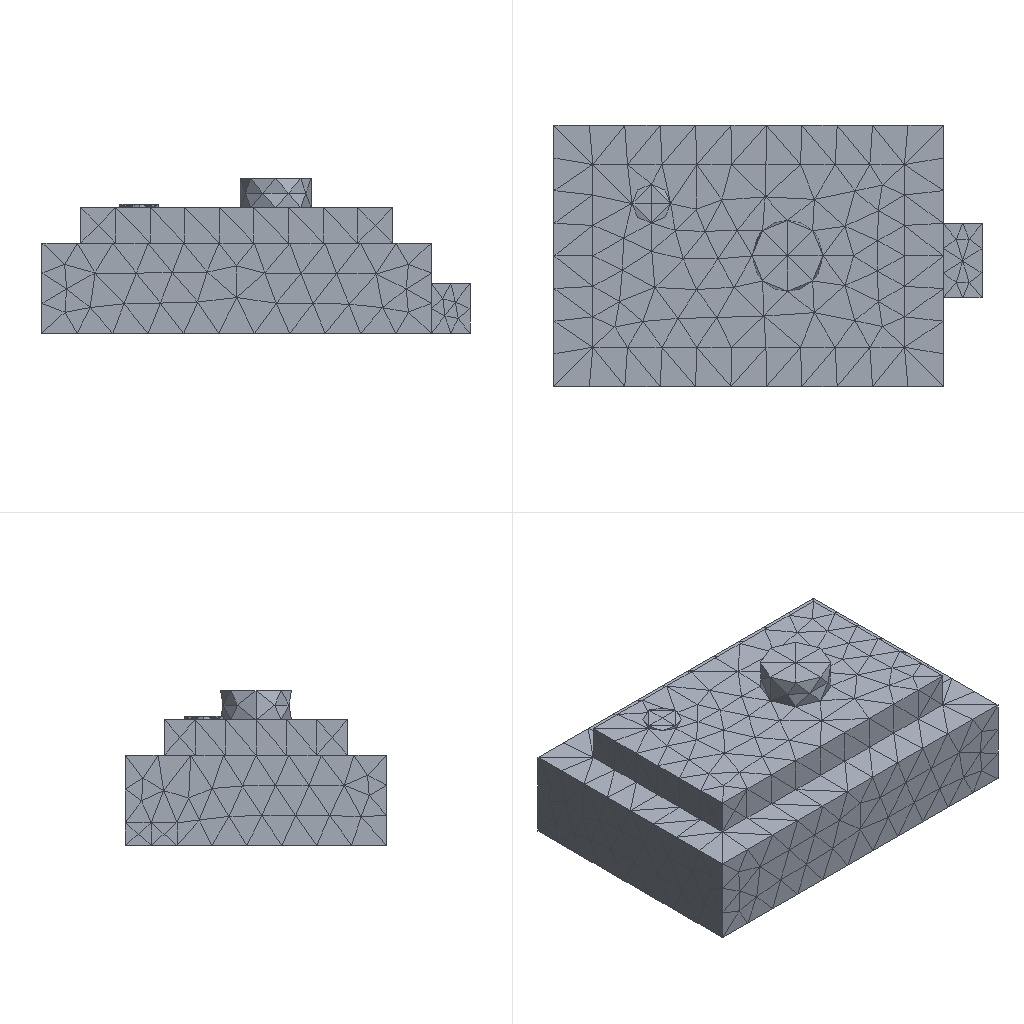Simulation study | ansys mapdl
Set-up summary:
category,name,step,type,value,unit,region
solver,ansys_mapdl
units,mm-N-s-tonne (MPa),,inferred,E=210000 density=
analysis,model,,static
mesh,nodes,,,4806
mesh,elements,,,2881
element_type,SOLID187,,,2881
material,mat 1,,E,210000
material,mat 1,,nu,0.3
load,,model,body load temp,,,all
load,,model,force,"1000 [dir=(0, 0, -1) n=142]",,node list
bc,,model,fixed,"[dofs=UX,UY,UZ n=5105]",,node list
Ansys APDL input file, long lists of numbers shortened:
/COM,ANSYS RELEASE 2026 R1           BUILD 26.1      UP20260202       09:09:57
/PREP7
/NOPR
/TITLE,2
ANTYPE, 0
*IF,_CDRDOFF,EQ,1,THEN     !if solid model was read in
_CDRDOFF=             !reset flag, numoffs already performed
*ELSE              !offset database for the following FE model
NUMOFF,NODE,     4806
NUMOFF,ELEM,     2881
NUMOFF,MAT ,        1
NUMOFF,TYPE,        1
*ENDIF
*SET,_RETURN ,  0.
*SET,_STATUS ,  0.
*SET,_UIQR   ,  142.
*SET,__FLOATPARAMETER__,  4806.
DOF,DELETE
ETBLOCK,        1,        1
(2i9,19a9)
        1      187        0        0        0        0        0        0        0        0        0        0        0        0        0        0        0        0        0        0        0
       -1
NBLOCK,6,SOLID,      4806,      4806
(3i9,6e21.13e3)
        1        0        0-4.4400000000000E+001 4.0500000000000E+001 7.0000000000000E+000
! (4805 more lines like these left out)
N,UNBL,LOC,       -1,
EBLOCK,19,SOLID,      2881,      2881
(19i10)
         1         1         1         1         0         0         0         0        10         0         1      1827       404      1828      1829      2104      2105      2106      2107
! (5761 more lines like these left out)
        -1
MPTEMP,UNBL, 1, 1,  0.    ,
MPDATA,UNBL, 1,EX  ,       1, 1,  210000.000    ,
MPTEMP,UNBL, 1, 1,  0.    ,
MPDATA,UNBL, 1,NUXY,       1, 1, 0.3    ,
MPTEMP,UNBL, 1, 1,  0.    ,
MPDATA,UNBL, 1,PRXY,       1, 1, 0.3    ,
EXTOPT,ATTR,      0,      0,      0
EXTOPT,ESIZE,  0,  0.
EXTOPT,ACLEAR,      0
TREF,  0.
IRLF,  0
BFUNIF,TEMP,_TINY
ACEL,  0.    ,  0.    ,  0.
OMEGA,  0.    ,  0.    ,  0.
DOMEGA,  0.    ,  0.    ,  0.
CGLOC,  0.    ,  0.    ,  0.
CGOMEGA,  0.    ,  0.    ,  0.
DCGOMG,  0.    ,  0.    ,  0.
KUSE,     0
TIME,  0.
ALPHAD,  0.
BETAD,  0.
DMPRAT,  0.
DMPSTR,  0.
CRPLIM, 0.1    ,   0
CRPLIM,  0.    ,   1
NCNV,     0, 1.000000000E+12,     0,  0.    ,  0.
NEQIT,     0
ERESX,DEFA
DBLOCK,      5105
(i9,a6,2(pg16.9))
        1  UX    0.00000000      0.00000000
! (5104 more lines like these left out)
       -1
FBLOCK,       142
(i9,a6,2(pg16.9))
      839  FZ   -7.04225352      0.00000000
! (141 more lines like these left out)
       -1
/GO
FINISH
Results summary:
result,analysis_type_db,,,static,unstated
result,n_sets,,,1,unstated
result,load_steps[0].set,load_step=1,,1,unstated
result,load_steps[0].substep,load_step=1,,1,unstated
result,load_steps[0].time,load_step=1,,1,unstated
result,load_steps[0].freq,load_step=1,,1,unstated
result,load_steps[0].max_usum,load_step=1,,0.0002603,unstated
result,load_steps[0].max_seqv,load_step=1,,23.345,unstated
result,load_steps[0].reaction_sum.FX,load_step=1,,4.31749e-12,unstated
result,load_steps[0].reaction_sum.FY,load_step=1,,-9.85736e-12,unstated
result,load_steps[0].reaction_sum.FZ,load_step=1,,1000,unstated
result,load_steps[0].reaction_sum.MX,load_step=1,,0,unstated
result,load_steps[0].reaction_sum.MY,load_step=1,,0,unstated
result,load_steps[0].reaction_sum.MZ,load_step=1,,0,unstated
result,convergence,,,results present for all listed sets,unstated